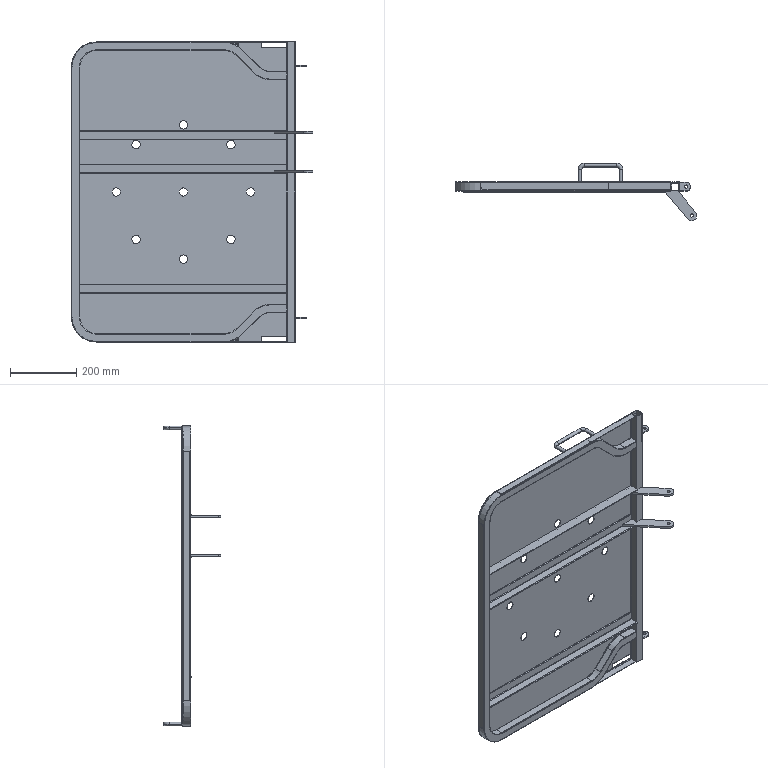Part | NX | features BREP 7 | 12 solids | 373 faces | box 731.436 x 173.677 x 910.59 mm | volume 1958159 mm3 | plane 186 | cylinder 147 | torus 32 | spline 8 | commonest cylinder face diameters 3.175 x47 25.4 x20 11.113 x12 10.998 x8 19.05 x8 1.587 x6